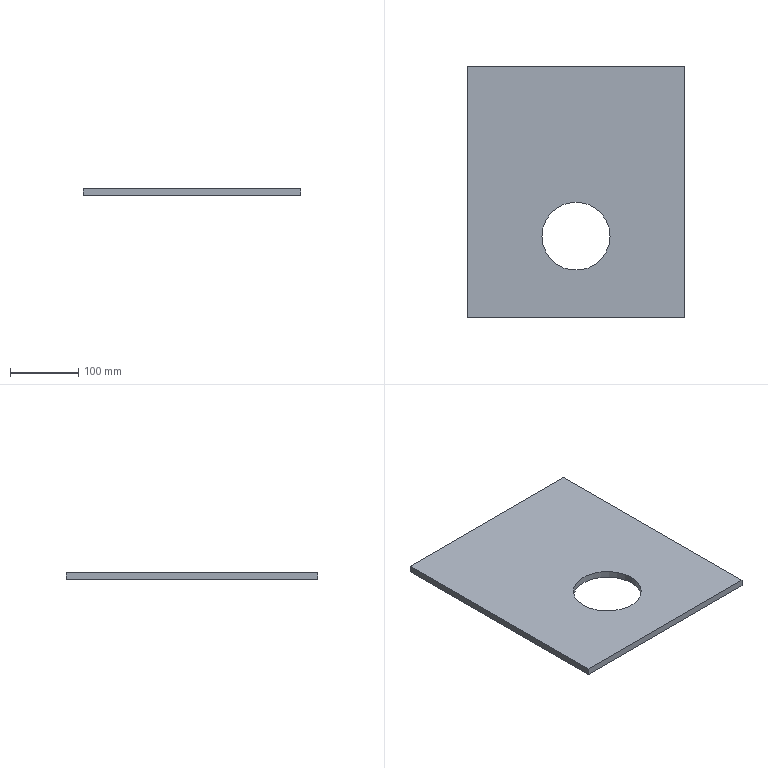Part | SolidWorks | features Extrusion 1 | 1 solid | 8 faces | box 320 x 370 x 10 mm | volume 1105460 mm3 | plane 6 | cylinder 2 | commonest cylinder face diameters 100 x2
STEP:
#1=CARTESIAN_POINT('',(110.,120.,10.));
#2=VERTEX_POINT('',#1);
#3=CARTESIAN_POINT('',(210.,120.,10.));
#4=VERTEX_POINT('',#3);
#5=CARTESIAN_POINT('',(160.,120.,10.));
#6=DIRECTION('',(0.,0.,1.));
#7=DIRECTION('',(1.,0.,0.));
#8=AXIS2_PLACEMENT_3D('',#5,#6,#7);
#9=CIRCLE('',#8,50.);
#10=EDGE_CURVE('',#2,#4,#9,.T.);
#11=ORIENTED_EDGE('',*,*,#10,.T.);
#12=CARTESIAN_POINT('',(210.,120.,0.));
#13=VERTEX_POINT('',#12);
#14=CARTESIAN_POINT('',(210.,120.,10.));
#15=DIRECTION('',(0.,0.,-1.));
#16=VECTOR('',#15,1000.);
#17=LINE('',#14,#16);
#18=EDGE_CURVE('',#4,#13,#17,.T.);
#19=ORIENTED_EDGE('',*,*,#18,.T.);
#20=CARTESIAN_POINT('',(110.,120.,0.));
#21=VERTEX_POINT('',#20);
#22=CARTESIAN_POINT('',(160.,120.,0.));
#23=DIRECTION('',(0.,0.,1.));
#24=DIRECTION('',(1.,0.,0.));
#25=AXIS2_PLACEMENT_3D('',#22,#23,#24);
#26=CIRCLE('',#25,50.);
#27=EDGE_CURVE('',#21,#13,#26,.T.);
#28=ORIENTED_EDGE('',*,*,#27,.F.);
#29=CARTESIAN_POINT('',(110.,120.,10.));
#30=DIRECTION('',(0.,0.,-1.));
#31=VECTOR('',#30,1000.);
#32=LINE('',#29,#31);
#33=EDGE_CURVE('',#2,#21,#32,.T.);
#34=ORIENTED_EDGE('',*,*,#33,.F.);
#35=EDGE_LOOP('',(#11,#19,#28,#34));
#36=FACE_OUTER_BOUND('',#35,.T.);
#37=CARTESIAN_POINT('',(160.,120.,10.));
#38=DIRECTION('',(0.,0.,-1.));
#39=DIRECTION('',(-1.,0.,0.));
#40=AXIS2_PLACEMENT_3D('',#37,#38,#39);
#41=CYLINDRICAL_SURFACE('',#40,50.);
#42=ADVANCED_FACE('',(#36),#41,.F.);
#43=CARTESIAN_POINT('',(0.,370.,10.));
#44=VERTEX_POINT('',#43);
#45=CARTESIAN_POINT('',(0.,0.,10.));
#46=VERTEX_POINT('',#45);
#47=CARTESIAN_POINT('',(0.,0.,10.));
#48=DIRECTION('',(0.,-1.,0.));
#49=VECTOR('',#48,1000.);
#50=LINE('',#47,#49);
#51=EDGE_CURVE('',#44,#46,#50,.T.);
#52=ORIENTED_EDGE('',*,*,#51,.T.);
#53=CARTESIAN_POINT('',(320.,0.,10.));
#54=VERTEX_POINT('',#53);
#55=CARTESIAN_POINT('',(0.,0.,10.));
#56=DIRECTION('',(1.,0.,0.));
#57=VECTOR('',#56,1000.);
#58=LINE('',#55,#57);
#59=EDGE_CURVE('',#46,#54,#58,.T.);
#60=ORIENTED_EDGE('',*,*,#59,.T.);
#61=CARTESIAN_POINT('',(320.,370.,10.));
#62=VERTEX_POINT('',#61);
#63=CARTESIAN_POINT('',(320.,0.,10.));
#64=DIRECTION('',(0.,1.,0.));
#65=VECTOR('',#64,1000.);
#66=LINE('',#63,#65);
#67=EDGE_CURVE('',#54,#62,#66,.T.);
#68=ORIENTED_EDGE('',*,*,#67,.T.);
#69=CARTESIAN_POINT('',(0.,370.,10.));
#70=DIRECTION('',(-1.,0.,0.));
#71=VECTOR('',#70,1000.);
#72=LINE('',#69,#71);
#73=EDGE_CURVE('',#62,#44,#72,.T.);
#74=ORIENTED_EDGE('',*,*,#73,.T.);
#75=EDGE_LOOP('',(#52,#60,#68,#74));
#76=FACE_OUTER_BOUND('',#75,.T.);
#77=ORIENTED_EDGE('',*,*,#10,.F.);
#78=CARTESIAN_POINT('',(160.,120.,10.));
#79=DIRECTION('',(0.,0.,1.));
#80=DIRECTION('',(1.,0.,0.));
#81=AXIS2_PLACEMENT_3D('',#78,#79,#80);
#82=CIRCLE('',#81,50.);
#83=EDGE_CURVE('',#4,#2,#82,.T.);
#84=ORIENTED_EDGE('',*,*,#83,.F.);
#85=EDGE_LOOP('',(#77,#84));
#86=FACE_BOUND('',#85,.T.);
#87=CARTESIAN_POINT('',(0.,370.,10.));
#88=DIRECTION('',(0.,0.,-1.));
#89=DIRECTION('',(-1.,0.,0.));
#90=AXIS2_PLACEMENT_3D('',#87,#88,#89);
#91=PLANE('',#90);
#92=ADVANCED_FACE('',(#76,#86),#91,.F.);
#93=CARTESIAN_POINT('',(0.,370.,0.));
#94=VERTEX_POINT('',#93);
#95=CARTESIAN_POINT('',(0.,0.,0.));
#96=VERTEX_POINT('',#95);
#97=CARTESIAN_POINT('',(0.,0.,0.));
#98=DIRECTION('',(0.,-1.,0.));
#99=VECTOR('',#98,1000.);
#100=LINE('',#97,#99);
#101=EDGE_CURVE('',#94,#96,#100,.T.);
#102=ORIENTED_EDGE('',*,*,#101,.F.);
#103=CARTESIAN_POINT('',(320.,370.,0.));
#104=VERTEX_POINT('',#103);
#105=CARTESIAN_POINT('',(0.,370.,0.));
#106=DIRECTION('',(-1.,0.,0.));
#107=VECTOR('',#106,1000.);
#108=LINE('',#105,#107);
#109=EDGE_CURVE('',#104,#94,#108,.T.);
#110=ORIENTED_EDGE('',*,*,#109,.F.);
#111=CARTESIAN_POINT('',(320.,0.,0.));
#112=VERTEX_POINT('',#111);
#113=CARTESIAN_POINT('',(320.,0.,0.));
#114=DIRECTION('',(0.,1.,0.));
#115=VECTOR('',#114,1000.);
#116=LINE('',#113,#115);
#117=EDGE_CURVE('',#112,#104,#116,.T.);
#118=ORIENTED_EDGE('',*,*,#117,.F.);
#119=CARTESIAN_POINT('',(0.,0.,0.));
#120=DIRECTION('',(1.,0.,0.));
#121=VECTOR('',#120,1000.);
#122=LINE('',#119,#121);
#123=EDGE_CURVE('',#96,#112,#122,.T.);
#124=ORIENTED_EDGE('',*,*,#123,.F.);
#125=EDGE_LOOP('',(#102,#110,#118,#124));
#126=FACE_OUTER_BOUND('',#125,.T.);
#127=ORIENTED_EDGE('',*,*,#27,.T.);
#128=CARTESIAN_POINT('',(160.,120.,0.));
#129=DIRECTION('',(0.,0.,1.));
#130=DIRECTION('',(1.,0.,0.));
#131=AXIS2_PLACEMENT_3D('',#128,#129,#130);
#132=CIRCLE('',#131,50.);
#133=EDGE_CURVE('',#13,#21,#132,.T.);
#134=ORIENTED_EDGE('',*,*,#133,.T.);
#135=EDGE_LOOP('',(#127,#134));
#136=FACE_BOUND('',#135,.T.);
#137=CARTESIAN_POINT('',(0.,370.,0.));
#138=DIRECTION('',(0.,0.,-1.));
#139=DIRECTION('',(-1.,0.,0.));
#140=AXIS2_PLACEMENT_3D('',#137,#138,#139);
#141=PLANE('',#140);
#142=ADVANCED_FACE('',(#126,#136),#141,.T.);
#143=ORIENTED_EDGE('',*,*,#101,.T.);
#144=CARTESIAN_POINT('',(0.,0.,10.));
#145=DIRECTION('',(0.,0.,-1.));
#146=VECTOR('',#145,1000.);
#147=LINE('',#144,#146);
#148=EDGE_CURVE('',#46,#96,#147,.T.);
#149=ORIENTED_EDGE('',*,*,#148,.F.);
#150=ORIENTED_EDGE('',*,*,#51,.F.);
#151=CARTESIAN_POINT('',(0.,370.,10.));
#152=DIRECTION('',(0.,0.,-1.));
#153=VECTOR('',#152,1000.);
#154=LINE('',#151,#153);
#155=EDGE_CURVE('',#44,#94,#154,.T.);
#156=ORIENTED_EDGE('',*,*,#155,.T.);
#157=EDGE_LOOP('',(#143,#149,#150,#156));
#158=FACE_OUTER_BOUND('',#157,.T.);
#159=CARTESIAN_POINT('',(0.,0.,10.));
#160=DIRECTION('',(1.,0.,0.));
#161=DIRECTION('',(0.,0.,-1.));
#162=AXIS2_PLACEMENT_3D('',#159,#160,#161);
#163=PLANE('',#162);
#164=ADVANCED_FACE('',(#158),#163,.F.);
#165=ORIENTED_EDGE('',*,*,#123,.T.);
#166=CARTESIAN_POINT('',(320.,0.,10.));
#167=DIRECTION('',(0.,0.,-1.));
#168=VECTOR('',#167,1000.);
#169=LINE('',#166,#168);
#170=EDGE_CURVE('',#54,#112,#169,.T.);
#171=ORIENTED_EDGE('',*,*,#170,.F.);
#172=ORIENTED_EDGE('',*,*,#59,.F.);
#173=ORIENTED_EDGE('',*,*,#148,.T.);
#174=EDGE_LOOP('',(#165,#171,#172,#173));
#175=FACE_OUTER_BOUND('',#174,.T.);
#176=CARTESIAN_POINT('',(0.,0.,10.));
#177=DIRECTION('',(0.,1.,0.));
#178=DIRECTION('',(0.,0.,1.));
#179=AXIS2_PLACEMENT_3D('',#176,#177,#178);
#180=PLANE('',#179);
#181=ADVANCED_FACE('',(#175),#180,.F.);
#182=ORIENTED_EDGE('',*,*,#117,.T.);
#183=CARTESIAN_POINT('',(320.,370.,10.));
#184=DIRECTION('',(0.,0.,-1.));
#185=VECTOR('',#184,1000.);
#186=LINE('',#183,#185);
#187=EDGE_CURVE('',#62,#104,#186,.T.);
#188=ORIENTED_EDGE('',*,*,#187,.F.);
#189=ORIENTED_EDGE('',*,*,#67,.F.);
#190=ORIENTED_EDGE('',*,*,#170,.T.);
#191=EDGE_LOOP('',(#182,#188,#189,#190));
#192=FACE_OUTER_BOUND('',#191,.T.);
#193=CARTESIAN_POINT('',(320.,0.,10.));
#194=DIRECTION('',(-1.,0.,0.));
#195=DIRECTION('',(0.,0.,1.));
#196=AXIS2_PLACEMENT_3D('',#193,#194,#195);
#197=PLANE('',#196);
#198=ADVANCED_FACE('',(#192),#197,.F.);
#199=ORIENTED_EDGE('',*,*,#109,.T.);
#200=ORIENTED_EDGE('',*,*,#155,.F.);
#201=ORIENTED_EDGE('',*,*,#73,.F.);
#202=ORIENTED_EDGE('',*,*,#187,.T.);
#203=EDGE_LOOP('',(#199,#200,#201,#202));
#204=FACE_OUTER_BOUND('',#203,.T.);
#205=CARTESIAN_POINT('',(0.,370.,10.));
#206=DIRECTION('',(0.,-1.,0.));
#207=DIRECTION('',(0.,0.,-1.));
#208=AXIS2_PLACEMENT_3D('',#205,#206,#207);
#209=PLANE('',#208);
#210=ADVANCED_FACE('',(#204),#209,.F.);
#211=ORIENTED_EDGE('',*,*,#18,.F.);
#212=ORIENTED_EDGE('',*,*,#83,.T.);
#213=ORIENTED_EDGE('',*,*,#33,.T.);
#214=ORIENTED_EDGE('',*,*,#133,.F.);
#215=EDGE_LOOP('',(#211,#212,#213,#214));
#216=FACE_OUTER_BOUND('',#215,.T.);
#217=CARTESIAN_POINT('',(160.,120.,10.));
#218=DIRECTION('',(0.,0.,-1.));
#219=DIRECTION('',(-1.,0.,0.));
#220=AXIS2_PLACEMENT_3D('',#217,#218,#219);
#221=CYLINDRICAL_SURFACE('',#220,50.);
#222=ADVANCED_FACE('',(#216),#221,.F.);
#223=CLOSED_SHELL('',(#42,#92,#142,#164,#181,#198,#210,#222));
#224=MANIFOLD_SOLID_BREP('',#223);
#225=CARTESIAN_POINT('',(0.,0.,0.));
#226=DIRECTION('',(0.,0.,1.));
#227=DIRECTION('',(1.,0.,0.));
#228=AXIS2_PLACEMENT_3D('',#225,#226,#227);
#229=(LENGTH_UNIT()NAMED_UNIT(*)SI_UNIT(.MILLI.,.METRE.));
#230=UNCERTAINTY_MEASURE_WITH_UNIT(LENGTH_MEASURE(0.00001),#229,'','');
#231=(NAMED_UNIT(*)PLANE_ANGLE_UNIT()SI_UNIT($,.RADIAN.));
#232=(NAMED_UNIT(*)SI_UNIT($,.STERADIAN.)SOLID_ANGLE_UNIT());
#233=(GEOMETRIC_REPRESENTATION_CONTEXT(3)GLOBAL_UNCERTAINTY_ASSIGNED_CONTEXT((#230))GLOBAL_UNIT_ASSIGNED_CONTEXT((#229,#231,#232))REPRESENTATION_CONTEXT('',''));
#234=ADVANCED_BREP_SHAPE_REPRESENTATION('',(#224,#228),#233);